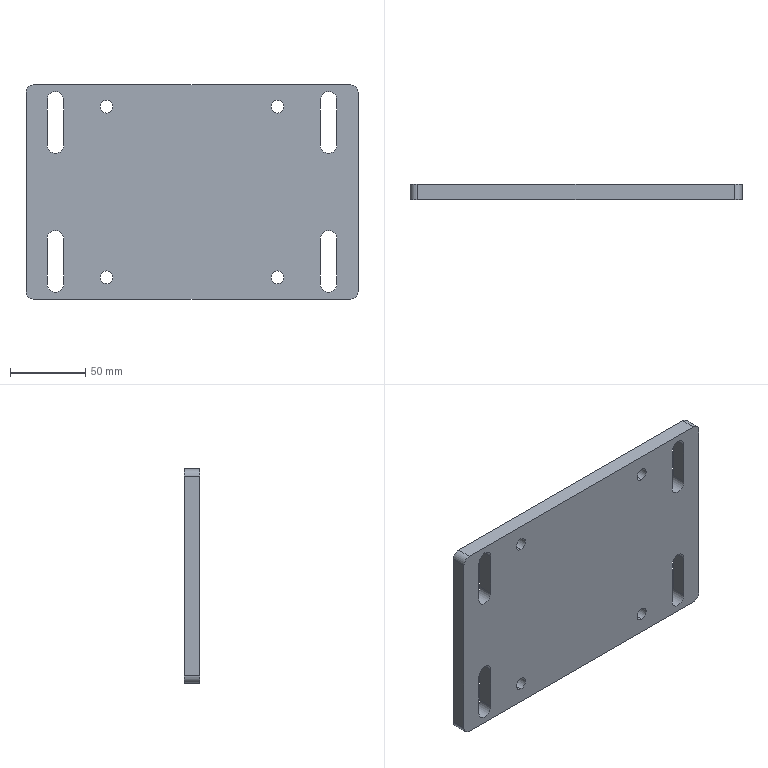Part | STEP file | 3-Motor plate | 1 solid | 38 faces | box 220 x 10 x 142 mm | volume 292914 mm3 | cylinder 24 | plane 14 | commonest cylinder face diameters 11 x12 8.5 x8 10 x4